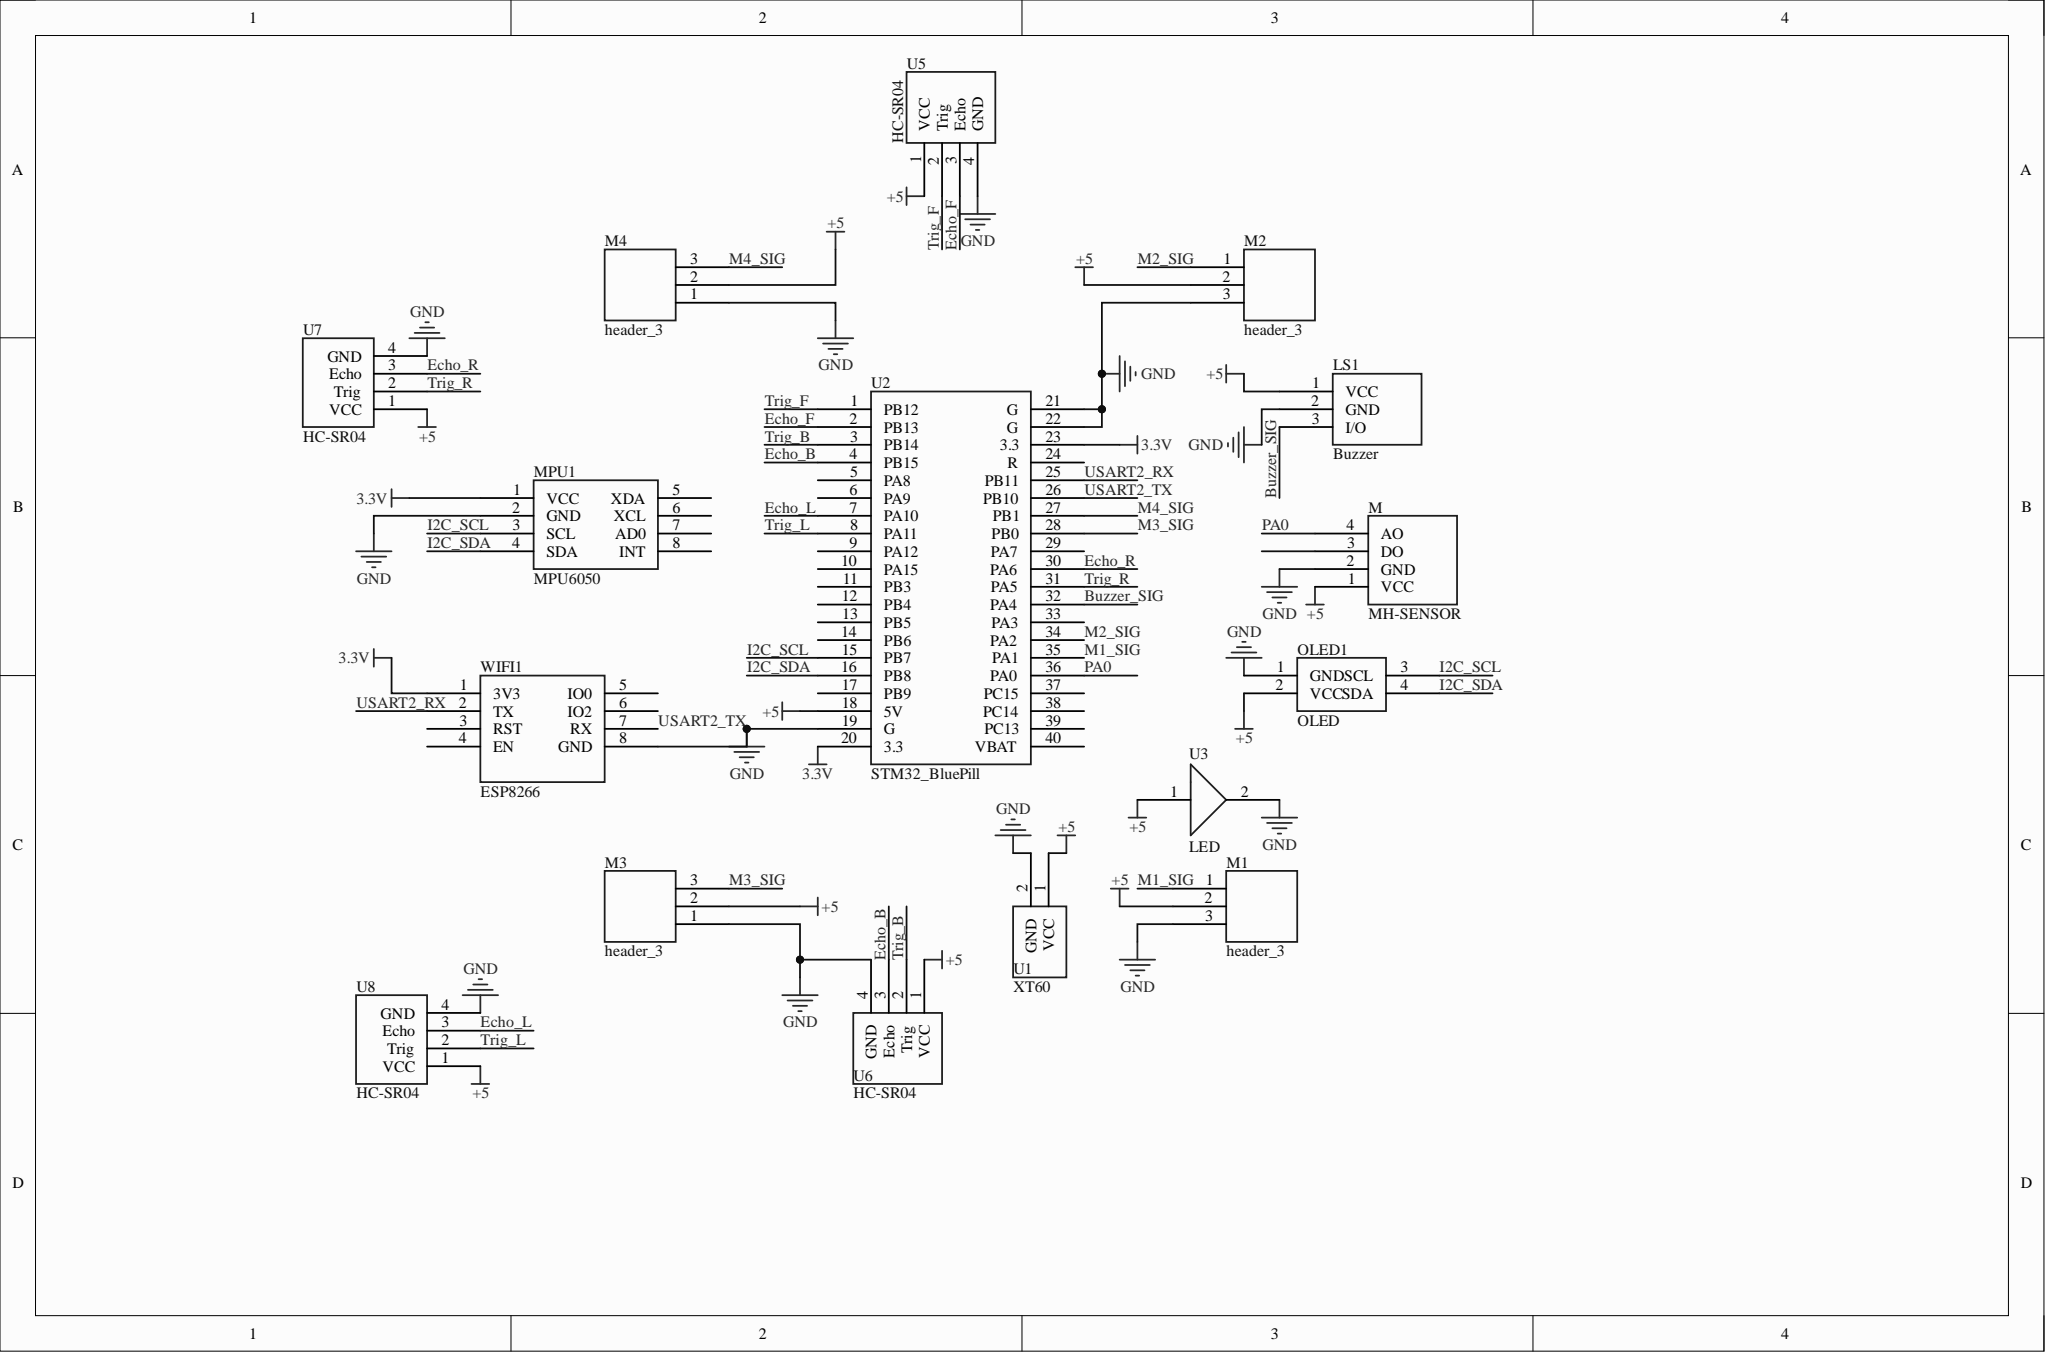Circuit board | Altium Designer | 16 parts | 21 nets
Bill of materials:
Comment,Description,Designator,Footprint,LibRef,Quantity
"Buzzer","","LS1","header","Buzzer","1"
"MH-SENSOR","","M","OLED","MH-SENSOR","1"
"header_3","","M1, M2, M3, M4","header","header_3","4"
"MPU6050","","MPU1","MPU6050","MPU6050_1","1"
"OLED","","OLED1","OLED","OLED_3","1"
"XT60","","U1","XT60","XT60_2","1"
"STM32_BluePill","","U2","STM32_BluePill_1","STM32_BluePill","1"
"LED","","U3","XT60","LED","1"
"HC-SR04","","U5, U6, U7, U8","OLED","HC-SR04, HC-SR04_1","4"
"ESP8266","","WIFI1","ESP8266","ESP8266_1","1"
Netlist (Protel format):
[
LS1
header
Buzzer



]
[
M
OLED
MH-SENSOR



]
[
M1
header
header_3



]
[
M2
header
header_3



]
[
M3
header
header_3



]
[
M4
header
header_3



]
[
MPU1
MPU6050
MPU6050



]
[
OLED1
OLED
OLED



]
[
U1
XT60
XT60



]
[
U2
STM32_BluePill_1
STM32_BluePill



]
[
U3
XT60
LED



]
[
U5
OLED
HC-SR04



]
[
U6
OLED
HC-SR04



]
[
U7
OLED
HC-SR04



]
[
U8
OLED
HC-SR04



]
[
WIFI1
ESP8266
ESP8266



]
(
USART2_TX
U2-26
WIFI1-7
)
(
USART2_RX
U2-25
WIFI1-2
)
(
Trig_R
U2-31
U7-2
)
(
Trig_L
U2-8
U8-2
)
(
Trig_F
U2-1
U5-2
)
(
Trig_B
U2-3
U6-2
)
(
PA0
M-4
U2-36
)
(
M4_SIG
M4-3
U2-27
)
(
M3_SIG
M3-3
U2-28
)
(
M2_SIG
M2-1
U2-34
)
(
M1_SIG
M1-1
U2-35
)
(
I2C_SDA
MPU1-4
OLED1-4
U2-16
)
(
I2C_SCL
MPU1-3
OLED1-3
U2-15
)
(
GND
LS1-2
M-2
M1-3
M2-3
M3-1
M4-1
MPU1-2
OLED1-1
U1-2
U2-19
U2-21
U2-22
U3-2
U5-4
U6-4
U7-4
U8-4
WIFI1-8
)
(
Echo_R
U2-30
U7-3
)
(
Echo_L
U2-7
U8-3
)
(
Echo_F
U2-2
U5-3
)
(
Echo_B
U2-4
U6-3
)
(
Buzzer_SIG
LS1-3
U2-32
)
(
+5
LS1-1
M-1
M1-2
M2-2
M3-2
M4-2
OLED1-2
U1-1
U2-18
U3-1
U5-1
U6-1
U7-1
U8-1
)
(
3.3V
MPU1-1
U2-20
U2-23
WIFI1-1
)